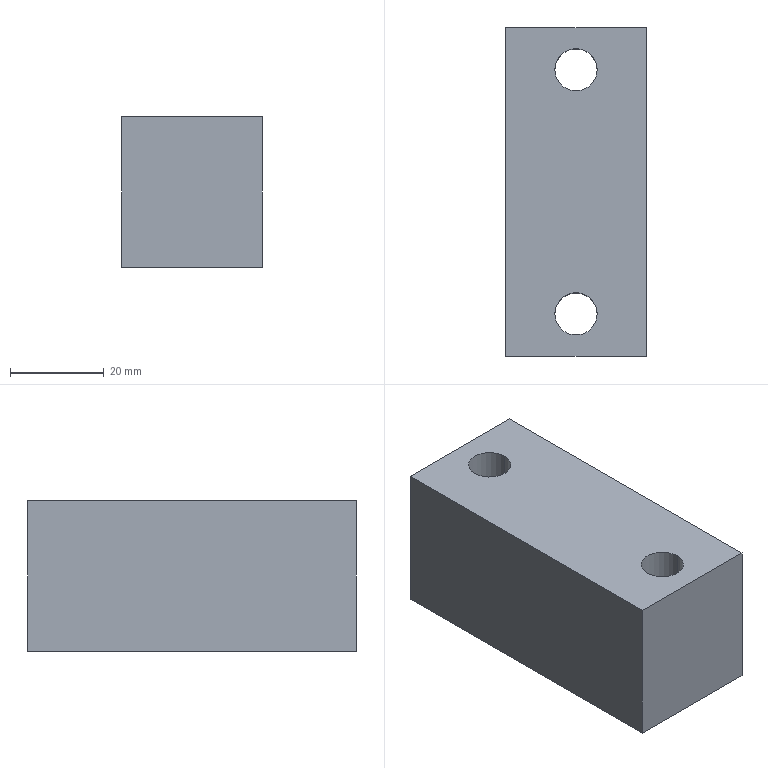Part | STEP file | X77-04006 | 1 solid | 10 faces | box 30 x 70 x 32 mm | volume 63128 mm3 | plane 6 | cylinder 4 | commonest cylinder face diameters 9 x4
STEP:
#1=CARTESIAN_POINT('',(-322.5,17.349,0.));
#2=VERTEX_POINT('',#1);
#3=CARTESIAN_POINT('',(-313.5,17.349,0.));
#4=VERTEX_POINT('',#3);
#5=CARTESIAN_POINT('',(-318.,17.349,0.));
#6=DIRECTION('',(0.,0.,1.));
#7=DIRECTION('',(1.,0.,0.));
#8=AXIS2_PLACEMENT_3D('',#5,#6,#7);
#9=CIRCLE('',#8,4.5);
#10=EDGE_CURVE('',#2,#4,#9,.T.);
#11=ORIENTED_EDGE('',*,*,#10,.F.);
#12=CARTESIAN_POINT('',(-322.5,17.349,32.));
#13=VERTEX_POINT('',#12);
#14=CARTESIAN_POINT('',(-322.5,17.349,0.));
#15=DIRECTION('',(0.,0.,1.));
#16=VECTOR('',#15,1000.);
#17=LINE('',#14,#16);
#18=EDGE_CURVE('',#2,#13,#17,.T.);
#19=ORIENTED_EDGE('',*,*,#18,.T.);
#20=CARTESIAN_POINT('',(-313.5,17.349,32.));
#21=VERTEX_POINT('',#20);
#22=CARTESIAN_POINT('',(-318.,17.349,32.));
#23=DIRECTION('',(0.,0.,1.));
#24=DIRECTION('',(1.,0.,0.));
#25=AXIS2_PLACEMENT_3D('',#22,#23,#24);
#26=CIRCLE('',#25,4.5);
#27=EDGE_CURVE('',#13,#21,#26,.T.);
#28=ORIENTED_EDGE('',*,*,#27,.T.);
#29=CARTESIAN_POINT('',(-313.5,17.349,0.));
#30=DIRECTION('',(0.,0.,1.));
#31=VECTOR('',#30,1000.);
#32=LINE('',#29,#31);
#33=EDGE_CURVE('',#4,#21,#32,.T.);
#34=ORIENTED_EDGE('',*,*,#33,.F.);
#35=EDGE_LOOP('',(#11,#19,#28,#34));
#36=FACE_OUTER_BOUND('',#35,.T.);
#37=CARTESIAN_POINT('',(-318.,17.349,0.));
#38=DIRECTION('',(0.,0.,1.));
#39=DIRECTION('',(1.,0.,0.));
#40=AXIS2_PLACEMENT_3D('',#37,#38,#39);
#41=CYLINDRICAL_SURFACE('',#40,4.5);
#42=ADVANCED_FACE('',(#36),#41,.F.);
#43=CARTESIAN_POINT('',(-322.5,69.349,0.));
#44=VERTEX_POINT('',#43);
#45=CARTESIAN_POINT('',(-313.5,69.349,0.));
#46=VERTEX_POINT('',#45);
#47=CARTESIAN_POINT('',(-318.,69.349,0.));
#48=DIRECTION('',(0.,0.,1.));
#49=DIRECTION('',(1.,0.,0.));
#50=AXIS2_PLACEMENT_3D('',#47,#48,#49);
#51=CIRCLE('',#50,4.5);
#52=EDGE_CURVE('',#44,#46,#51,.T.);
#53=ORIENTED_EDGE('',*,*,#52,.F.);
#54=CARTESIAN_POINT('',(-322.5,69.349,32.));
#55=VERTEX_POINT('',#54);
#56=CARTESIAN_POINT('',(-322.5,69.349,0.));
#57=DIRECTION('',(0.,0.,1.));
#58=VECTOR('',#57,1000.);
#59=LINE('',#56,#58);
#60=EDGE_CURVE('',#44,#55,#59,.T.);
#61=ORIENTED_EDGE('',*,*,#60,.T.);
#62=CARTESIAN_POINT('',(-313.5,69.349,32.));
#63=VERTEX_POINT('',#62);
#64=CARTESIAN_POINT('',(-318.,69.349,32.));
#65=DIRECTION('',(0.,0.,1.));
#66=DIRECTION('',(1.,0.,0.));
#67=AXIS2_PLACEMENT_3D('',#64,#65,#66);
#68=CIRCLE('',#67,4.5);
#69=EDGE_CURVE('',#55,#63,#68,.T.);
#70=ORIENTED_EDGE('',*,*,#69,.T.);
#71=CARTESIAN_POINT('',(-313.5,69.349,0.));
#72=DIRECTION('',(0.,0.,1.));
#73=VECTOR('',#72,1000.);
#74=LINE('',#71,#73);
#75=EDGE_CURVE('',#46,#63,#74,.T.);
#76=ORIENTED_EDGE('',*,*,#75,.F.);
#77=EDGE_LOOP('',(#53,#61,#70,#76));
#78=FACE_OUTER_BOUND('',#77,.T.);
#79=CARTESIAN_POINT('',(-318.,69.349,0.));
#80=DIRECTION('',(0.,0.,1.));
#81=DIRECTION('',(1.,0.,0.));
#82=AXIS2_PLACEMENT_3D('',#79,#80,#81);
#83=CYLINDRICAL_SURFACE('',#82,4.5);
#84=ADVANCED_FACE('',(#78),#83,.F.);
#85=CARTESIAN_POINT('',(-303.,78.349,0.));
#86=VERTEX_POINT('',#85);
#87=CARTESIAN_POINT('',(-333.,78.349,0.));
#88=VERTEX_POINT('',#87);
#89=CARTESIAN_POINT('',(-333.,78.349,0.));
#90=DIRECTION('',(-1.,0.,0.));
#91=VECTOR('',#90,1000.);
#92=LINE('',#89,#91);
#93=EDGE_CURVE('',#86,#88,#92,.T.);
#94=ORIENTED_EDGE('',*,*,#93,.T.);
#95=CARTESIAN_POINT('',(-333.,78.349,32.));
#96=VERTEX_POINT('',#95);
#97=CARTESIAN_POINT('',(-333.,78.349,32.));
#98=DIRECTION('',(0.,0.,-1.));
#99=VECTOR('',#98,1000.);
#100=LINE('',#97,#99);
#101=EDGE_CURVE('',#96,#88,#100,.T.);
#102=ORIENTED_EDGE('',*,*,#101,.F.);
#103=CARTESIAN_POINT('',(-303.,78.349,32.));
#104=VERTEX_POINT('',#103);
#105=CARTESIAN_POINT('',(-333.,78.349,32.));
#106=DIRECTION('',(-1.,0.,0.));
#107=VECTOR('',#106,1000.);
#108=LINE('',#105,#107);
#109=EDGE_CURVE('',#104,#96,#108,.T.);
#110=ORIENTED_EDGE('',*,*,#109,.F.);
#111=CARTESIAN_POINT('',(-303.,78.349,32.));
#112=DIRECTION('',(0.,0.,-1.));
#113=VECTOR('',#112,1000.);
#114=LINE('',#111,#113);
#115=EDGE_CURVE('',#104,#86,#114,.T.);
#116=ORIENTED_EDGE('',*,*,#115,.T.);
#117=EDGE_LOOP('',(#94,#102,#110,#116));
#118=FACE_OUTER_BOUND('',#117,.T.);
#119=CARTESIAN_POINT('',(-333.,78.349,32.));
#120=DIRECTION('',(0.,-1.,0.));
#121=DIRECTION('',(0.,0.,-1.));
#122=AXIS2_PLACEMENT_3D('',#119,#120,#121);
#123=PLANE('',#122);
#124=ADVANCED_FACE('',(#118),#123,.F.);
#125=CARTESIAN_POINT('',(-333.,8.349,0.));
#126=VERTEX_POINT('',#125);
#127=CARTESIAN_POINT('',(-333.,78.349,0.));
#128=DIRECTION('',(0.,-1.,0.));
#129=VECTOR('',#128,1000.);
#130=LINE('',#127,#129);
#131=EDGE_CURVE('',#88,#126,#130,.T.);
#132=ORIENTED_EDGE('',*,*,#131,.T.);
#133=CARTESIAN_POINT('',(-333.,8.349,32.));
#134=VERTEX_POINT('',#133);
#135=CARTESIAN_POINT('',(-333.,8.349,32.));
#136=DIRECTION('',(0.,0.,-1.));
#137=VECTOR('',#136,1000.);
#138=LINE('',#135,#137);
#139=EDGE_CURVE('',#134,#126,#138,.T.);
#140=ORIENTED_EDGE('',*,*,#139,.F.);
#141=CARTESIAN_POINT('',(-333.,78.349,32.));
#142=DIRECTION('',(0.,-1.,0.));
#143=VECTOR('',#142,1000.);
#144=LINE('',#141,#143);
#145=EDGE_CURVE('',#96,#134,#144,.T.);
#146=ORIENTED_EDGE('',*,*,#145,.F.);
#147=ORIENTED_EDGE('',*,*,#101,.T.);
#148=EDGE_LOOP('',(#132,#140,#146,#147));
#149=FACE_OUTER_BOUND('',#148,.T.);
#150=CARTESIAN_POINT('',(-333.,78.349,32.));
#151=DIRECTION('',(1.,0.,0.));
#152=DIRECTION('',(0.,0.,-1.));
#153=AXIS2_PLACEMENT_3D('',#150,#151,#152);
#154=PLANE('',#153);
#155=ADVANCED_FACE('',(#149),#154,.F.);
#156=CARTESIAN_POINT('',(-303.,8.349,0.));
#157=VERTEX_POINT('',#156);
#158=CARTESIAN_POINT('',(-333.,8.349,0.));
#159=DIRECTION('',(1.,0.,0.));
#160=VECTOR('',#159,1000.);
#161=LINE('',#158,#160);
#162=EDGE_CURVE('',#126,#157,#161,.T.);
#163=ORIENTED_EDGE('',*,*,#162,.T.);
#164=CARTESIAN_POINT('',(-303.,8.349,32.));
#165=VERTEX_POINT('',#164);
#166=CARTESIAN_POINT('',(-303.,8.349,32.));
#167=DIRECTION('',(0.,0.,-1.));
#168=VECTOR('',#167,1000.);
#169=LINE('',#166,#168);
#170=EDGE_CURVE('',#165,#157,#169,.T.);
#171=ORIENTED_EDGE('',*,*,#170,.F.);
#172=CARTESIAN_POINT('',(-333.,8.349,32.));
#173=DIRECTION('',(1.,0.,0.));
#174=VECTOR('',#173,1000.);
#175=LINE('',#172,#174);
#176=EDGE_CURVE('',#134,#165,#175,.T.);
#177=ORIENTED_EDGE('',*,*,#176,.F.);
#178=ORIENTED_EDGE('',*,*,#139,.T.);
#179=EDGE_LOOP('',(#163,#171,#177,#178));
#180=FACE_OUTER_BOUND('',#179,.T.);
#181=CARTESIAN_POINT('',(-333.,8.349,32.));
#182=DIRECTION('',(0.,1.,0.));
#183=DIRECTION('',(-1.,0.,0.));
#184=AXIS2_PLACEMENT_3D('',#181,#182,#183);
#185=PLANE('',#184);
#186=ADVANCED_FACE('',(#180),#185,.F.);
#187=CARTESIAN_POINT('',(-303.,78.349,0.));
#188=DIRECTION('',(0.,1.,0.));
#189=VECTOR('',#188,1000.);
#190=LINE('',#187,#189);
#191=EDGE_CURVE('',#157,#86,#190,.T.);
#192=ORIENTED_EDGE('',*,*,#191,.T.);
#193=ORIENTED_EDGE('',*,*,#115,.F.);
#194=CARTESIAN_POINT('',(-303.,78.349,32.));
#195=DIRECTION('',(0.,1.,0.));
#196=VECTOR('',#195,1000.);
#197=LINE('',#194,#196);
#198=EDGE_CURVE('',#165,#104,#197,.T.);
#199=ORIENTED_EDGE('',*,*,#198,.F.);
#200=ORIENTED_EDGE('',*,*,#170,.T.);
#201=EDGE_LOOP('',(#192,#193,#199,#200));
#202=FACE_OUTER_BOUND('',#201,.T.);
#203=CARTESIAN_POINT('',(-303.,78.349,32.));
#204=DIRECTION('',(-1.,0.,0.));
#205=DIRECTION('',(0.,0.,1.));
#206=AXIS2_PLACEMENT_3D('',#203,#204,#205);
#207=PLANE('',#206);
#208=ADVANCED_FACE('',(#202),#207,.F.);
#209=CARTESIAN_POINT('',(-318.,17.349,32.));
#210=DIRECTION('',(0.,0.,1.));
#211=DIRECTION('',(1.,0.,0.));
#212=AXIS2_PLACEMENT_3D('',#209,#210,#211);
#213=CIRCLE('',#212,4.5);
#214=EDGE_CURVE('',#21,#13,#213,.T.);
#215=ORIENTED_EDGE('',*,*,#214,.F.);
#216=ORIENTED_EDGE('',*,*,#27,.F.);
#217=EDGE_LOOP('',(#215,#216));
#218=FACE_BOUND('',#217,.T.);
#219=CARTESIAN_POINT('',(-318.,69.349,32.));
#220=DIRECTION('',(0.,0.,1.));
#221=DIRECTION('',(1.,0.,0.));
#222=AXIS2_PLACEMENT_3D('',#219,#220,#221);
#223=CIRCLE('',#222,4.5);
#224=EDGE_CURVE('',#63,#55,#223,.T.);
#225=ORIENTED_EDGE('',*,*,#224,.F.);
#226=ORIENTED_EDGE('',*,*,#69,.F.);
#227=EDGE_LOOP('',(#225,#226));
#228=FACE_BOUND('',#227,.T.);
#229=ORIENTED_EDGE('',*,*,#109,.T.);
#230=ORIENTED_EDGE('',*,*,#145,.T.);
#231=ORIENTED_EDGE('',*,*,#176,.T.);
#232=ORIENTED_EDGE('',*,*,#198,.T.);
#233=EDGE_LOOP('',(#229,#230,#231,#232));
#234=FACE_OUTER_BOUND('',#233,.T.);
#235=CARTESIAN_POINT('',(-303.,78.349,32.));
#236=DIRECTION('',(0.,0.,-1.));
#237=DIRECTION('',(-1.,0.,0.));
#238=AXIS2_PLACEMENT_3D('',#235,#236,#237);
#239=PLANE('',#238);
#240=ADVANCED_FACE('',(#218,#228,#234),#239,.F.);
#241=CARTESIAN_POINT('',(-318.,17.349,0.));
#242=DIRECTION('',(0.,0.,1.));
#243=DIRECTION('',(1.,0.,0.));
#244=AXIS2_PLACEMENT_3D('',#241,#242,#243);
#245=CIRCLE('',#244,4.5);
#246=EDGE_CURVE('',#4,#2,#245,.T.);
#247=ORIENTED_EDGE('',*,*,#246,.T.);
#248=ORIENTED_EDGE('',*,*,#10,.T.);
#249=EDGE_LOOP('',(#247,#248));
#250=FACE_BOUND('',#249,.T.);
#251=CARTESIAN_POINT('',(-318.,69.349,0.));
#252=DIRECTION('',(0.,0.,1.));
#253=DIRECTION('',(1.,0.,0.));
#254=AXIS2_PLACEMENT_3D('',#251,#252,#253);
#255=CIRCLE('',#254,4.5);
#256=EDGE_CURVE('',#46,#44,#255,.T.);
#257=ORIENTED_EDGE('',*,*,#256,.T.);
#258=ORIENTED_EDGE('',*,*,#52,.T.);
#259=EDGE_LOOP('',(#257,#258));
#260=FACE_BOUND('',#259,.T.);
#261=ORIENTED_EDGE('',*,*,#93,.F.);
#262=ORIENTED_EDGE('',*,*,#191,.F.);
#263=ORIENTED_EDGE('',*,*,#162,.F.);
#264=ORIENTED_EDGE('',*,*,#131,.F.);
#265=EDGE_LOOP('',(#261,#262,#263,#264));
#266=FACE_OUTER_BOUND('',#265,.T.);
#267=CARTESIAN_POINT('',(-303.,78.349,0.));
#268=DIRECTION('',(0.,0.,-1.));
#269=DIRECTION('',(-1.,0.,0.));
#270=AXIS2_PLACEMENT_3D('',#267,#268,#269);
#271=PLANE('',#270);
#272=ADVANCED_FACE('',(#250,#260,#266),#271,.T.);
#273=ORIENTED_EDGE('',*,*,#60,.F.);
#274=ORIENTED_EDGE('',*,*,#256,.F.);
#275=ORIENTED_EDGE('',*,*,#75,.T.);
#276=ORIENTED_EDGE('',*,*,#224,.T.);
#277=EDGE_LOOP('',(#273,#274,#275,#276));
#278=FACE_OUTER_BOUND('',#277,.T.);
#279=CARTESIAN_POINT('',(-318.,69.349,0.));
#280=DIRECTION('',(0.,0.,1.));
#281=DIRECTION('',(1.,0.,0.));
#282=AXIS2_PLACEMENT_3D('',#279,#280,#281);
#283=CYLINDRICAL_SURFACE('',#282,4.5);
#284=ADVANCED_FACE('',(#278),#283,.F.);
#285=ORIENTED_EDGE('',*,*,#18,.F.);
#286=ORIENTED_EDGE('',*,*,#246,.F.);
#287=ORIENTED_EDGE('',*,*,#33,.T.);
#288=ORIENTED_EDGE('',*,*,#214,.T.);
#289=EDGE_LOOP('',(#285,#286,#287,#288));
#290=FACE_OUTER_BOUND('',#289,.T.);
#291=CARTESIAN_POINT('',(-318.,17.349,0.));
#292=DIRECTION('',(0.,0.,1.));
#293=DIRECTION('',(1.,0.,0.));
#294=AXIS2_PLACEMENT_3D('',#291,#292,#293);
#295=CYLINDRICAL_SURFACE('',#294,4.5);
#296=ADVANCED_FACE('',(#290),#295,.F.);
#297=CLOSED_SHELL('',(#42,#84,#124,#155,#186,#208,#240,#272,#284,#296));
#298=MANIFOLD_SOLID_BREP('',#297);
#299=CARTESIAN_POINT('',(0.,0.,0.));
#300=DIRECTION('',(0.,0.,1.));
#301=DIRECTION('',(1.,0.,0.));
#302=AXIS2_PLACEMENT_3D('',#299,#300,#301);
#303=(LENGTH_UNIT()NAMED_UNIT(*)SI_UNIT(.MILLI.,.METRE.));
#304=UNCERTAINTY_MEASURE_WITH_UNIT(LENGTH_MEASURE(0.00001),#303,'','');
#305=(NAMED_UNIT(*)PLANE_ANGLE_UNIT()SI_UNIT($,.RADIAN.));
#306=(NAMED_UNIT(*)SI_UNIT($,.STERADIAN.)SOLID_ANGLE_UNIT());
#307=(GEOMETRIC_REPRESENTATION_CONTEXT(3)GLOBAL_UNCERTAINTY_ASSIGNED_CONTEXT((#304))GLOBAL_UNIT_ASSIGNED_CONTEXT((#303,#305,#306))REPRESENTATION_CONTEXT('',''));
#308=ADVANCED_BREP_SHAPE_REPRESENTATION('',(#298,#302),#307);